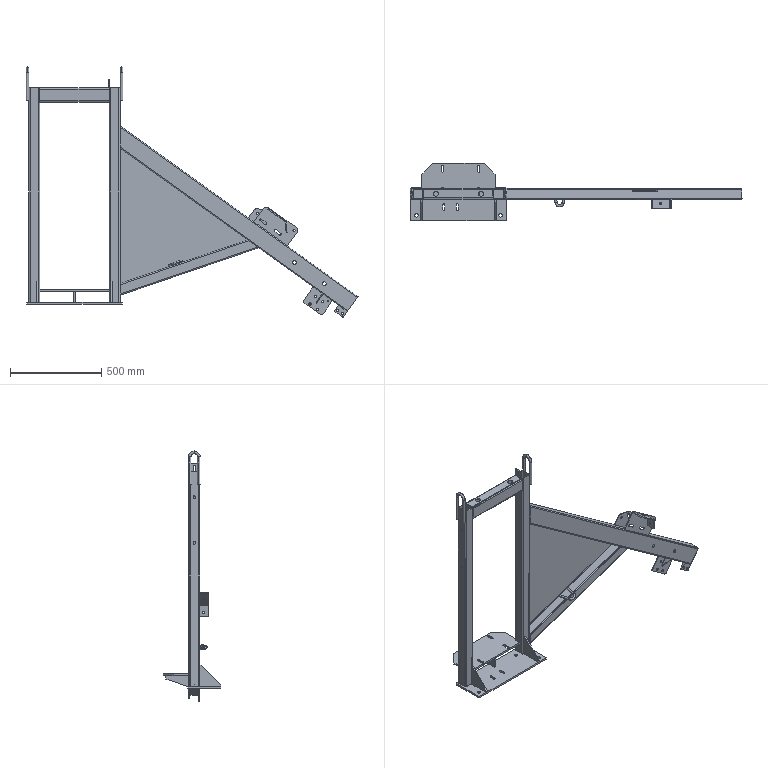Part | SolidWorks | features ICE 15, Cut 6, WeldCornerFeat 4, WeldMemberFeat 4, 3DProfileFeature 3, Gusset 3, HoleWzd 3, Sweep 2, Extrusion 1, Fillet 1, FlatPattern 1, MirrorSolid 1, MoveCopyBody 1, SM3dBend 1, SMBaseFlange 1, SheetMetal 1, WeldmentFeature 1 | 21 solids | 364 faces | box 1815 x 315 x 1367 mm | volume 6905440 mm3 | plane 201 | cylinder 153 | torus 10 | commonest cylinder face diameters 12 x33 14 x16 16 x14 8 x12 13 x12 20 x10